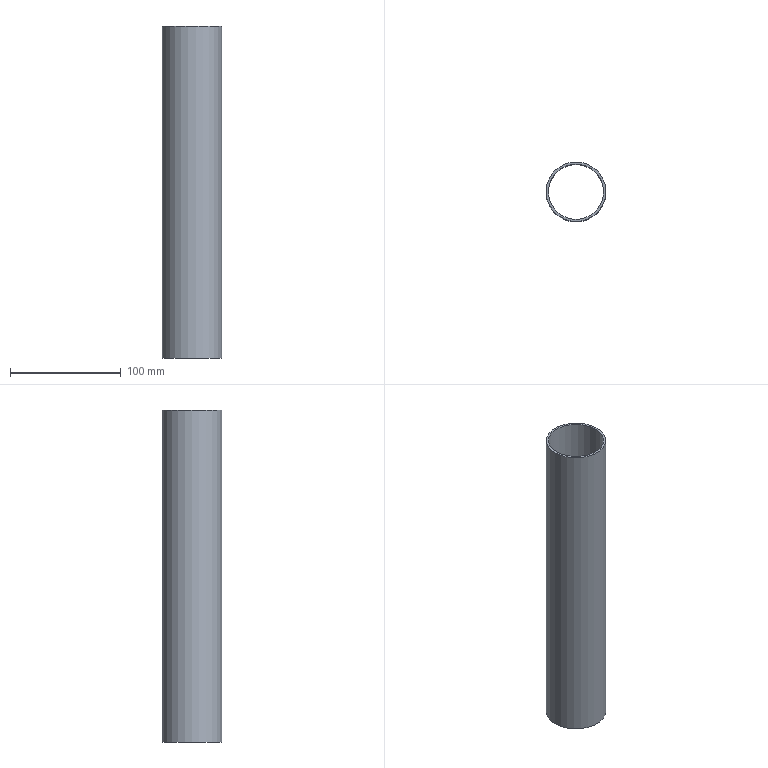Part | STEP file | JBJ-P-1012-01 | 1 solid | 4 faces | box 54 x 54 x 300 mm | volume 98018 mm3 | cylinder 2 | plane 2 | commonest cylinder face diameters 50 x1 54 x1
STEP:
#1=CARTESIAN_POINT('',(325.,0.,-350.));
#2=VERTEX_POINT('',#1);
#3=CARTESIAN_POINT('',(350.,0.,-350.));
#4=DIRECTION('',(0.,0.,-1.));
#5=DIRECTION('',(-1.,0.,0.));
#6=AXIS2_PLACEMENT_3D('',#3,#4,#5);
#7=CIRCLE('',#6,25.);
#8=EDGE_CURVE('',#2,#2,#7,.T.);
#9=ORIENTED_EDGE('',*,*,#8,.F.);
#10=EDGE_LOOP('',(#9));
#11=FACE_OUTER_BOUND('',#10,.T.);
#12=CARTESIAN_POINT('',(325.,0.,-650.));
#13=VERTEX_POINT('',#12);
#14=CARTESIAN_POINT('',(350.,0.,-650.));
#15=DIRECTION('',(0.,0.,1.));
#16=DIRECTION('',(-1.,0.,0.));
#17=AXIS2_PLACEMENT_3D('',#14,#15,#16);
#18=CIRCLE('',#17,25.);
#19=EDGE_CURVE('',#13,#13,#18,.T.);
#20=ORIENTED_EDGE('',*,*,#19,.F.);
#21=EDGE_LOOP('',(#20));
#22=FACE_OUTER_BOUND('',#21,.T.);
#23=CARTESIAN_POINT('',(350.,0.,-250.));
#24=DIRECTION('',(0.,0.,-1.));
#25=DIRECTION('',(-1.,0.,0.));
#26=AXIS2_PLACEMENT_3D('',#23,#24,#25);
#27=CYLINDRICAL_SURFACE('',#26,25.);
#28=ADVANCED_FACE('',(#11,#22),#27,.F.);
#29=ORIENTED_EDGE('',*,*,#19,.T.);
#30=EDGE_LOOP('',(#29));
#31=FACE_BOUND('',#30,.T.);
#32=CARTESIAN_POINT('',(323.,0.,-650.));
#33=VERTEX_POINT('',#32);
#34=CARTESIAN_POINT('',(350.,0.,-650.));
#35=DIRECTION('',(0.,0.,-1.));
#36=DIRECTION('',(-1.,0.,0.));
#37=AXIS2_PLACEMENT_3D('',#34,#35,#36);
#38=CIRCLE('',#37,27.);
#39=EDGE_CURVE('',#33,#33,#38,.T.);
#40=ORIENTED_EDGE('',*,*,#39,.T.);
#41=EDGE_LOOP('',(#40));
#42=FACE_OUTER_BOUND('',#41,.T.);
#43=CARTESIAN_POINT('',(350.,0.,-650.));
#44=DIRECTION('',(0.,0.,-1.));
#45=DIRECTION('',(-1.,0.,0.));
#46=AXIS2_PLACEMENT_3D('',#43,#44,#45);
#47=PLANE('',#46);
#48=ADVANCED_FACE('',(#31,#42),#47,.T.);
#49=CARTESIAN_POINT('',(323.,0.,-350.));
#50=VERTEX_POINT('',#49);
#51=CARTESIAN_POINT('',(350.,0.,-350.));
#52=DIRECTION('',(0.,0.,1.));
#53=DIRECTION('',(-1.,0.,0.));
#54=AXIS2_PLACEMENT_3D('',#51,#52,#53);
#55=CIRCLE('',#54,27.);
#56=EDGE_CURVE('',#50,#50,#55,.T.);
#57=ORIENTED_EDGE('',*,*,#56,.F.);
#58=EDGE_LOOP('',(#57));
#59=FACE_OUTER_BOUND('',#58,.T.);
#60=ORIENTED_EDGE('',*,*,#39,.F.);
#61=EDGE_LOOP('',(#60));
#62=FACE_OUTER_BOUND('',#61,.T.);
#63=CARTESIAN_POINT('',(350.,0.,-250.));
#64=DIRECTION('',(0.,0.,-1.));
#65=DIRECTION('',(-1.,0.,0.));
#66=AXIS2_PLACEMENT_3D('',#63,#64,#65);
#67=CYLINDRICAL_SURFACE('',#66,27.);
#68=ADVANCED_FACE('',(#59,#62),#67,.T.);
#69=ORIENTED_EDGE('',*,*,#56,.T.);
#70=EDGE_LOOP('',(#69));
#71=FACE_OUTER_BOUND('',#70,.T.);
#72=ORIENTED_EDGE('',*,*,#8,.T.);
#73=EDGE_LOOP('',(#72));
#74=FACE_BOUND('',#73,.T.);
#75=CARTESIAN_POINT('',(-10.,-27.,-350.));
#76=DIRECTION('',(0.,0.,-1.));
#77=DIRECTION('',(-1.,0.,0.));
#78=AXIS2_PLACEMENT_3D('',#75,#76,#77);
#79=PLANE('',#78);
#80=ADVANCED_FACE('',(#71,#74),#79,.F.);
#81=CLOSED_SHELL('',(#28,#48,#68,#80));
#82=MANIFOLD_SOLID_BREP('',#81);
#83=CARTESIAN_POINT('',(0.,0.,0.));
#84=DIRECTION('',(0.,0.,1.));
#85=DIRECTION('',(1.,0.,0.));
#86=AXIS2_PLACEMENT_3D('',#83,#84,#85);
#87=(LENGTH_UNIT()NAMED_UNIT(*)SI_UNIT(.MILLI.,.METRE.));
#88=UNCERTAINTY_MEASURE_WITH_UNIT(LENGTH_MEASURE(0.00001),#87,'','');
#89=(NAMED_UNIT(*)PLANE_ANGLE_UNIT()SI_UNIT($,.RADIAN.));
#90=(NAMED_UNIT(*)SI_UNIT($,.STERADIAN.)SOLID_ANGLE_UNIT());
#91=(GEOMETRIC_REPRESENTATION_CONTEXT(3)GLOBAL_UNCERTAINTY_ASSIGNED_CONTEXT((#88))GLOBAL_UNIT_ASSIGNED_CONTEXT((#87,#89,#90))REPRESENTATION_CONTEXT('',''));
#92=ADVANCED_BREP_SHAPE_REPRESENTATION('',(#82,#86),#91);